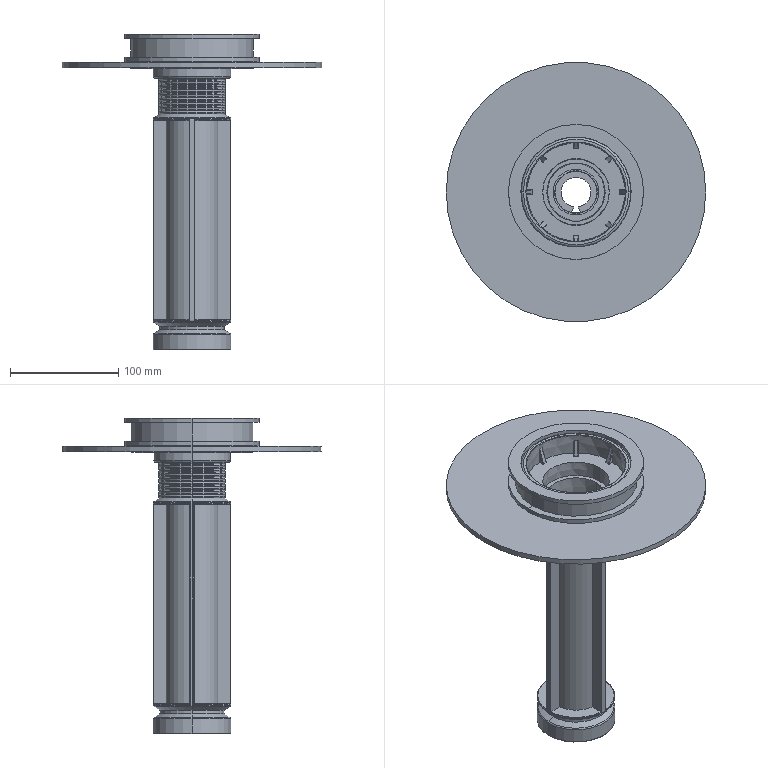Part | SolidWorks | features MoveCopyBody 2, MBimport 1, MoveFace 1 | 3 solids | 271 faces | box 240 x 240 x 292.1 mm | volume 610223 mm3 | cylinder 107 | torus 72 | plane 48 | cone 40 | spline 4 | commonest cylinder face diameters 60.4 x46 1 x28 42.38 x4 48 x4 72 x4 125 x4